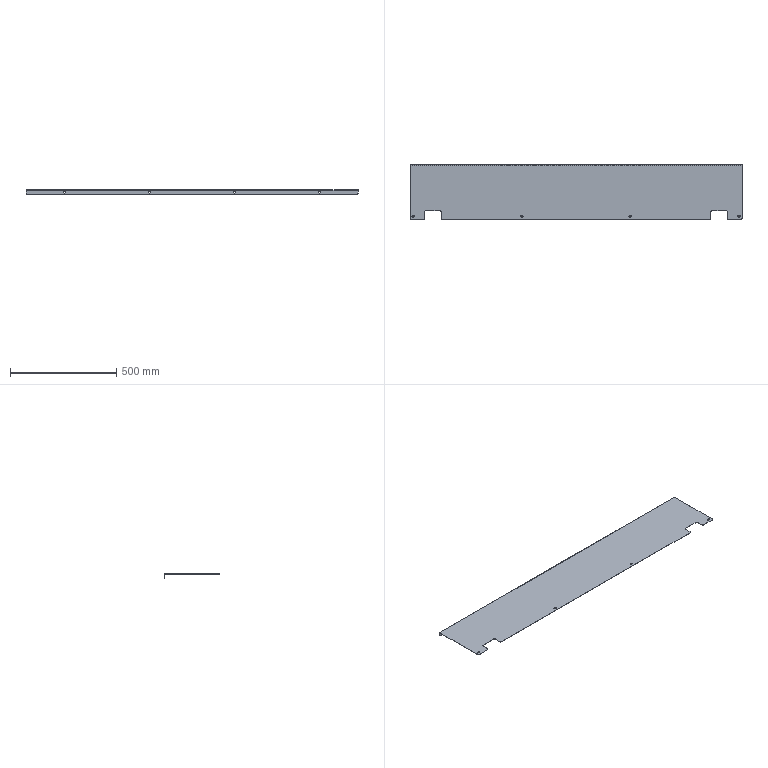Part | SolidWorks | features BaseBody 1 | 1 solid | 78 faces | box 1560 x 258.1 x 20 mm | volume 508789 mm3 | plane 52 | cylinder 26 | commonest cylinder face diameters 7 x12 10 x12 2 x1 4.4 x1